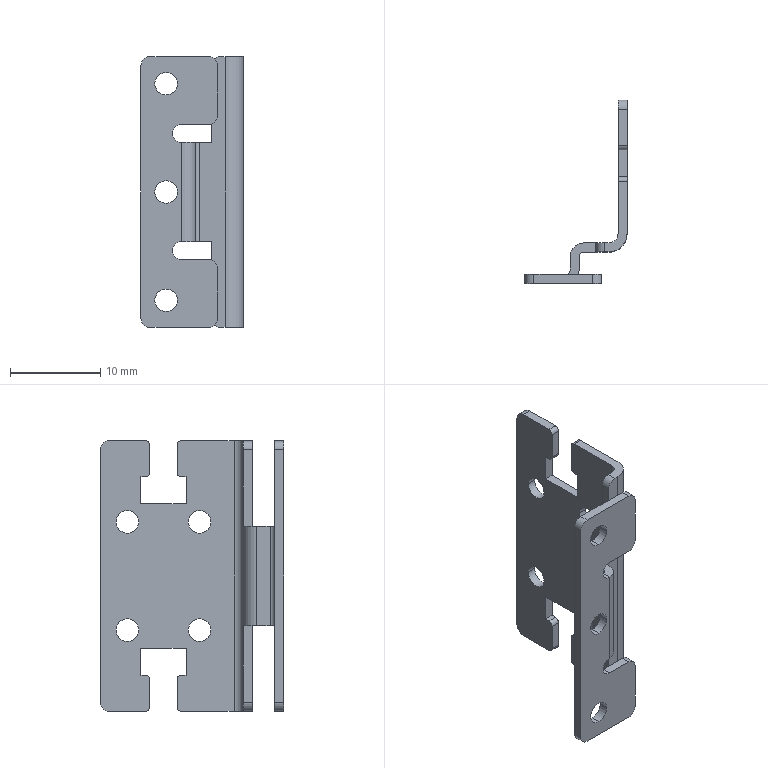Part | SolidWorks | features BaseBody 1 | 1 solid | 80 faces | box 11.322 x 20.322 x 30 mm | volume 726.14 mm3 | cylinder 42 | plane 38 | commonest cylinder face diameters 2 x15 2.5 x14 1 x10 3 x2 4 x1